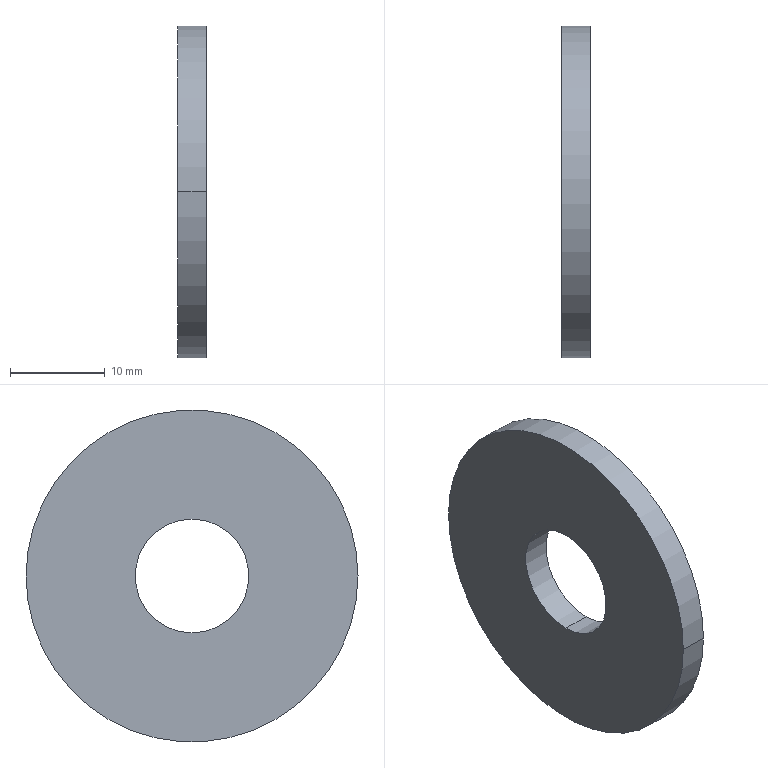Part | STEP file | [02]-15 | 1 solid | 6 faces | box 3 x 35 x 35 mm | volume 2547 mm3 | cylinder 4 | plane 2 | commonest cylinder face diameters 12 x2 35 x2
STEP:
#1=CARTESIAN_POINT('',(0.,0.,0.));
#2=DIRECTION('',(0.,0.,1.));
#3=DIRECTION('',(1.,0.,0.));
#4=AXIS2_PLACEMENT_3D('',#1,#2,#3);
#5=CARTESIAN_POINT('',(0.,0.,-6.));
#6=VERTEX_POINT('',#5);
#7=CARTESIAN_POINT('',(3.,0.,-6.));
#8=VERTEX_POINT('',#7);
#9=CARTESIAN_POINT('',(0.,0.,-6.));
#10=DIRECTION('',(1.,0.,0.));
#11=VECTOR('',#10,1.);
#12=LINE('',#9,#11);
#13=CARTESIAN_POINT('',(0.,0.,0.));
#14=DIRECTION('',(1.,0.,0.));
#15=DIRECTION('',(0.,0.,-1.));
#16=AXIS2_PLACEMENT_3D('',#13,#14,#15);
#17=CYLINDRICAL_SURFACE('',#16,6.);
#18=CARTESIAN_POINT('',(6.283,0.));
#19=DIRECTION('',(0.,1.));
#20=VECTOR('',#19,1.);
#21=LINE('',#18,#20);
#22=(GEOMETRIC_REPRESENTATION_CONTEXT(2)PARAMETRIC_REPRESENTATION_CONTEXT()REPRESENTATION_CONTEXT('',''));
#23=DEFINITIONAL_REPRESENTATION('',(#21),#22);
#24=PCURVE('',#17,#23);
#25=CARTESIAN_POINT('',(0.,0.,0.));
#26=DIRECTION('',(1.,0.,0.));
#27=DIRECTION('',(0.,0.,-1.));
#28=AXIS2_PLACEMENT_3D('',#25,#26,#27);
#29=CYLINDRICAL_SURFACE('',#28,6.);
#30=CARTESIAN_POINT('',(0.,0.));
#31=DIRECTION('',(0.,1.));
#32=VECTOR('',#31,1.);
#33=LINE('',#30,#32);
#34=(GEOMETRIC_REPRESENTATION_CONTEXT(2)PARAMETRIC_REPRESENTATION_CONTEXT()REPRESENTATION_CONTEXT('',''));
#35=DEFINITIONAL_REPRESENTATION('',(#33),#34);
#36=PCURVE('',#29,#35);
#37=SURFACE_CURVE('',#12,(#24,#36),.PCURVE_S1.);
#38=EDGE_CURVE('',#6,#8,#37,.T.);
#39=ORIENTED_EDGE('',*,*,#38,.T.);
#40=CARTESIAN_POINT('',(3.,0.,6.));
#41=VERTEX_POINT('',#40);
#42=CARTESIAN_POINT('',(3.,0.,0.));
#43=DIRECTION('',(-1.,0.,0.));
#44=DIRECTION('',(0.,0.,1.));
#45=AXIS2_PLACEMENT_3D('',#42,#43,#44);
#46=CIRCLE('',#45,6.);
#47=CARTESIAN_POINT('',(9.425,3.));
#48=DIRECTION('',(-1.,0.));
#49=VECTOR('',#48,1.);
#50=LINE('',#47,#49);
#51=(GEOMETRIC_REPRESENTATION_CONTEXT(2)PARAMETRIC_REPRESENTATION_CONTEXT()REPRESENTATION_CONTEXT('',''));
#52=DEFINITIONAL_REPRESENTATION('',(#50),#51);
#53=PCURVE('',#17,#52);
#54=CARTESIAN_POINT('',(3.,0.,0.));
#55=DIRECTION('',(1.,0.,0.));
#56=DIRECTION('',(0.,1.,0.));
#57=AXIS2_PLACEMENT_3D('',#54,#55,#56);
#58=PLANE('',#57);
#59=CARTESIAN_POINT('',(0.,6.));
#60=CARTESIAN_POINT('',(10.392,6.));
#61=CARTESIAN_POINT('',(5.196,-3.));
#62=CARTESIAN_POINT('',(0.,-12.));
#63=CARTESIAN_POINT('',(-5.196,-3.));
#64=CARTESIAN_POINT('',(-10.392,6.));
#65=CARTESIAN_POINT('',(0.,6.));
#66=(BOUNDED_CURVE()B_SPLINE_CURVE(2,(#59,#60,#61,#62,#63,#64,#65),.UNSPECIFIED.,.T.,.F.)B_SPLINE_CURVE_WITH_KNOTS((1,2,2,2,2,1),(-2.094,0.,2.094,4.189,6.283,8.378),.UNSPECIFIED.)CURVE()GEOMETRIC_REPRESENTATION_ITEM()RATIONAL_B_SPLINE_CURVE((1.,0.5,1.,0.5,1.,0.5,1.))REPRESENTATION_ITEM(''));
#67=(GEOMETRIC_REPRESENTATION_CONTEXT(2)PARAMETRIC_REPRESENTATION_CONTEXT()REPRESENTATION_CONTEXT('',''));
#68=DEFINITIONAL_REPRESENTATION('',(#66),#67);
#69=PCURVE('',#58,#68);
#70=SURFACE_CURVE('',#46,(#53,#69),.PCURVE_S1.);
#71=EDGE_CURVE('',#8,#41,#70,.T.);
#72=ORIENTED_EDGE('',*,*,#71,.T.);
#73=CARTESIAN_POINT('',(0.,0.,6.));
#74=VERTEX_POINT('',#73);
#75=CARTESIAN_POINT('',(0.,0.,6.));
#76=DIRECTION('',(1.,0.,0.));
#77=VECTOR('',#76,1.);
#78=LINE('',#75,#77);
#79=CARTESIAN_POINT('',(3.142,0.));
#80=DIRECTION('',(0.,1.));
#81=VECTOR('',#80,1.);
#82=LINE('',#79,#81);
#83=(GEOMETRIC_REPRESENTATION_CONTEXT(2)PARAMETRIC_REPRESENTATION_CONTEXT()REPRESENTATION_CONTEXT('',''));
#84=DEFINITIONAL_REPRESENTATION('',(#82),#83);
#85=PCURVE('',#17,#84);
#86=CARTESIAN_POINT('',(3.142,0.));
#87=DIRECTION('',(0.,1.));
#88=VECTOR('',#87,1.);
#89=LINE('',#86,#88);
#90=(GEOMETRIC_REPRESENTATION_CONTEXT(2)PARAMETRIC_REPRESENTATION_CONTEXT()REPRESENTATION_CONTEXT('',''));
#91=DEFINITIONAL_REPRESENTATION('',(#89),#90);
#92=PCURVE('',#29,#91);
#93=SURFACE_CURVE('',#78,(#85,#92),.PCURVE_S1.);
#94=EDGE_CURVE('',#74,#41,#93,.T.);
#95=ORIENTED_EDGE('',*,*,#94,.F.);
#96=CARTESIAN_POINT('',(0.,0.,0.));
#97=DIRECTION('',(1.,0.,0.));
#98=DIRECTION('',(0.,0.,-1.));
#99=AXIS2_PLACEMENT_3D('',#96,#97,#98);
#100=CIRCLE('',#99,6.);
#101=CARTESIAN_POINT('',(0.,0.));
#102=DIRECTION('',(1.,0.));
#103=VECTOR('',#102,1.);
#104=LINE('',#101,#103);
#105=(GEOMETRIC_REPRESENTATION_CONTEXT(2)PARAMETRIC_REPRESENTATION_CONTEXT()REPRESENTATION_CONTEXT('',''));
#106=DEFINITIONAL_REPRESENTATION('',(#104),#105);
#107=PCURVE('',#17,#106);
#108=CARTESIAN_POINT('',(0.,0.,0.));
#109=DIRECTION('',(-1.,0.,0.));
#110=DIRECTION('',(0.,-1.,0.));
#111=AXIS2_PLACEMENT_3D('',#108,#109,#110);
#112=PLANE('',#111);
#113=CARTESIAN_POINT('',(0.,-6.));
#114=CARTESIAN_POINT('',(-10.392,-6.));
#115=CARTESIAN_POINT('',(-5.196,3.));
#116=CARTESIAN_POINT('',(0.,12.));
#117=CARTESIAN_POINT('',(5.196,3.));
#118=CARTESIAN_POINT('',(10.392,-6.));
#119=CARTESIAN_POINT('',(0.,-6.));
#120=(BOUNDED_CURVE()B_SPLINE_CURVE(2,(#113,#114,#115,#116,#117,#118,#119),.UNSPECIFIED.,.T.,.F.)B_SPLINE_CURVE_WITH_KNOTS((1,2,2,2,2,1),(-2.094,0.,2.094,4.189,6.283,8.378),.UNSPECIFIED.)CURVE()GEOMETRIC_REPRESENTATION_ITEM()RATIONAL_B_SPLINE_CURVE((1.,0.5,1.,0.5,1.,0.5,1.))REPRESENTATION_ITEM(''));
#121=(GEOMETRIC_REPRESENTATION_CONTEXT(2)PARAMETRIC_REPRESENTATION_CONTEXT()REPRESENTATION_CONTEXT('',''));
#122=DEFINITIONAL_REPRESENTATION('',(#120),#121);
#123=PCURVE('',#112,#122);
#124=SURFACE_CURVE('',#100,(#107,#123),.PCURVE_S1.);
#125=EDGE_CURVE('',#74,#6,#124,.T.);
#126=ORIENTED_EDGE('',*,*,#125,.T.);
#127=EDGE_LOOP('',(#39,#72,#95,#126));
#128=FACE_BOUND('',#127,.F.);
#129=ADVANCED_FACE('',(#128),#17,.F.);
#130=CARTESIAN_POINT('',(0.,17.5,0.));
#131=VERTEX_POINT('',#130);
#132=CARTESIAN_POINT('',(0.,-17.5,0.));
#133=VERTEX_POINT('',#132);
#134=CARTESIAN_POINT('',(0.,0.,0.));
#135=DIRECTION('',(1.,0.,0.));
#136=DIRECTION('',(0.,1.,0.));
#137=AXIS2_PLACEMENT_3D('',#134,#135,#136);
#138=CIRCLE('',#137,17.5);
#139=CARTESIAN_POINT('',(0.,0.,0.));
#140=DIRECTION('',(1.,0.,0.));
#141=DIRECTION('',(0.,1.,0.));
#142=AXIS2_PLACEMENT_3D('',#139,#140,#141);
#143=CYLINDRICAL_SURFACE('',#142,17.5);
#144=CARTESIAN_POINT('',(0.,0.));
#145=DIRECTION('',(1.,0.));
#146=VECTOR('',#145,1.);
#147=LINE('',#144,#146);
#148=(GEOMETRIC_REPRESENTATION_CONTEXT(2)PARAMETRIC_REPRESENTATION_CONTEXT()REPRESENTATION_CONTEXT('',''));
#149=DEFINITIONAL_REPRESENTATION('',(#147),#148);
#150=PCURVE('',#143,#149);
#151=CARTESIAN_POINT('',(-17.5,0.));
#152=CARTESIAN_POINT('',(-17.5,30.311));
#153=CARTESIAN_POINT('',(8.75,15.155));
#154=CARTESIAN_POINT('',(35.,0.));
#155=CARTESIAN_POINT('',(8.75,-15.155));
#156=CARTESIAN_POINT('',(-17.5,-30.311));
#157=CARTESIAN_POINT('',(-17.5,0.));
#158=(BOUNDED_CURVE()B_SPLINE_CURVE(2,(#151,#152,#153,#154,#155,#156,#157),.UNSPECIFIED.,.T.,.F.)B_SPLINE_CURVE_WITH_KNOTS((1,2,2,2,2,1),(-2.094,0.,2.094,4.189,6.283,8.378),.UNSPECIFIED.)CURVE()GEOMETRIC_REPRESENTATION_ITEM()RATIONAL_B_SPLINE_CURVE((1.,0.5,1.,0.5,1.,0.5,1.))REPRESENTATION_ITEM(''));
#159=(GEOMETRIC_REPRESENTATION_CONTEXT(2)PARAMETRIC_REPRESENTATION_CONTEXT()REPRESENTATION_CONTEXT('',''));
#160=DEFINITIONAL_REPRESENTATION('',(#158),#159);
#161=PCURVE('',#112,#160);
#162=SURFACE_CURVE('',#138,(#150,#161),.PCURVE_S1.);
#163=EDGE_CURVE('',#131,#133,#162,.T.);
#164=ORIENTED_EDGE('',*,*,#163,.T.);
#165=CARTESIAN_POINT('',(3.,-17.5,0.));
#166=VERTEX_POINT('',#165);
#167=CARTESIAN_POINT('',(0.,-17.5,0.));
#168=DIRECTION('',(1.,0.,0.));
#169=VECTOR('',#168,1.);
#170=LINE('',#167,#169);
#171=CARTESIAN_POINT('',(3.142,0.));
#172=DIRECTION('',(0.,1.));
#173=VECTOR('',#172,1.);
#174=LINE('',#171,#173);
#175=(GEOMETRIC_REPRESENTATION_CONTEXT(2)PARAMETRIC_REPRESENTATION_CONTEXT()REPRESENTATION_CONTEXT('',''));
#176=DEFINITIONAL_REPRESENTATION('',(#174),#175);
#177=PCURVE('',#143,#176);
#178=CARTESIAN_POINT('',(0.,0.,0.));
#179=DIRECTION('',(1.,0.,0.));
#180=DIRECTION('',(0.,1.,0.));
#181=AXIS2_PLACEMENT_3D('',#178,#179,#180);
#182=CYLINDRICAL_SURFACE('',#181,17.5);
#183=CARTESIAN_POINT('',(3.142,0.));
#184=DIRECTION('',(0.,1.));
#185=VECTOR('',#184,1.);
#186=LINE('',#183,#185);
#187=(GEOMETRIC_REPRESENTATION_CONTEXT(2)PARAMETRIC_REPRESENTATION_CONTEXT()REPRESENTATION_CONTEXT('',''));
#188=DEFINITIONAL_REPRESENTATION('',(#186),#187);
#189=PCURVE('',#182,#188);
#190=SURFACE_CURVE('',#170,(#177,#189),.PCURVE_S1.);
#191=EDGE_CURVE('',#133,#166,#190,.T.);
#192=ORIENTED_EDGE('',*,*,#191,.T.);
#193=CARTESIAN_POINT('',(3.,17.5,0.));
#194=VERTEX_POINT('',#193);
#195=CARTESIAN_POINT('',(3.,0.,0.));
#196=DIRECTION('',(-1.,0.,0.));
#197=DIRECTION('',(0.,-1.,0.));
#198=AXIS2_PLACEMENT_3D('',#195,#196,#197);
#199=CIRCLE('',#198,17.5);
#200=CARTESIAN_POINT('',(3.142,3.));
#201=DIRECTION('',(-1.,0.));
#202=VECTOR('',#201,1.);
#203=LINE('',#200,#202);
#204=(GEOMETRIC_REPRESENTATION_CONTEXT(2)PARAMETRIC_REPRESENTATION_CONTEXT()REPRESENTATION_CONTEXT('',''));
#205=DEFINITIONAL_REPRESENTATION('',(#203),#204);
#206=PCURVE('',#143,#205);
#207=CARTESIAN_POINT('',(-17.5,0.));
#208=CARTESIAN_POINT('',(-17.5,30.311));
#209=CARTESIAN_POINT('',(8.75,15.155));
#210=CARTESIAN_POINT('',(35.,0.));
#211=CARTESIAN_POINT('',(8.75,-15.155));
#212=CARTESIAN_POINT('',(-17.5,-30.311));
#213=CARTESIAN_POINT('',(-17.5,0.));
#214=(BOUNDED_CURVE()B_SPLINE_CURVE(2,(#207,#208,#209,#210,#211,#212,#213),.UNSPECIFIED.,.T.,.F.)B_SPLINE_CURVE_WITH_KNOTS((1,2,2,2,2,1),(-2.094,0.,2.094,4.189,6.283,8.378),.UNSPECIFIED.)CURVE()GEOMETRIC_REPRESENTATION_ITEM()RATIONAL_B_SPLINE_CURVE((1.,0.5,1.,0.5,1.,0.5,1.))REPRESENTATION_ITEM(''));
#215=(GEOMETRIC_REPRESENTATION_CONTEXT(2)PARAMETRIC_REPRESENTATION_CONTEXT()REPRESENTATION_CONTEXT('',''));
#216=DEFINITIONAL_REPRESENTATION('',(#214),#215);
#217=PCURVE('',#58,#216);
#218=SURFACE_CURVE('',#199,(#206,#217),.PCURVE_S1.);
#219=EDGE_CURVE('',#166,#194,#218,.T.);
#220=ORIENTED_EDGE('',*,*,#219,.T.);
#221=CARTESIAN_POINT('',(0.,17.5,0.));
#222=DIRECTION('',(1.,0.,0.));
#223=VECTOR('',#222,1.);
#224=LINE('',#221,#223);
#225=CARTESIAN_POINT('',(0.,0.));
#226=DIRECTION('',(0.,1.));
#227=VECTOR('',#226,1.);
#228=LINE('',#225,#227);
#229=(GEOMETRIC_REPRESENTATION_CONTEXT(2)PARAMETRIC_REPRESENTATION_CONTEXT()REPRESENTATION_CONTEXT('',''));
#230=DEFINITIONAL_REPRESENTATION('',(#228),#229);
#231=PCURVE('',#143,#230);
#232=CARTESIAN_POINT('',(6.283,0.));
#233=DIRECTION('',(0.,1.));
#234=VECTOR('',#233,1.);
#235=LINE('',#232,#234);
#236=(GEOMETRIC_REPRESENTATION_CONTEXT(2)PARAMETRIC_REPRESENTATION_CONTEXT()REPRESENTATION_CONTEXT('',''));
#237=DEFINITIONAL_REPRESENTATION('',(#235),#236);
#238=PCURVE('',#182,#237);
#239=SURFACE_CURVE('',#224,(#231,#238),.PCURVE_S1.);
#240=EDGE_CURVE('',#131,#194,#239,.T.);
#241=ORIENTED_EDGE('',*,*,#240,.F.);
#242=EDGE_LOOP('',(#164,#192,#220,#241));
#243=FACE_BOUND('',#242,.T.);
#244=ADVANCED_FACE('',(#243),#143,.T.);
#245=ORIENTED_EDGE('',*,*,#71,.T.);
#246=CARTESIAN_POINT('',(3.,0.,0.));
#247=DIRECTION('',(-1.,0.,0.));
#248=DIRECTION('',(0.,0.,1.));
#249=AXIS2_PLACEMENT_3D('',#246,#247,#248);
#250=CIRCLE('',#249,6.);
#251=CARTESIAN_POINT('',(0.,6.));
#252=CARTESIAN_POINT('',(10.392,6.));
#253=CARTESIAN_POINT('',(5.196,-3.));
#254=CARTESIAN_POINT('',(0.,-12.));
#255=CARTESIAN_POINT('',(-5.196,-3.));
#256=CARTESIAN_POINT('',(-10.392,6.));
#257=CARTESIAN_POINT('',(0.,6.));
#258=(BOUNDED_CURVE()B_SPLINE_CURVE(2,(#251,#252,#253,#254,#255,#256,#257),.UNSPECIFIED.,.T.,.F.)B_SPLINE_CURVE_WITH_KNOTS((1,2,2,2,2,1),(-2.094,0.,2.094,4.189,6.283,8.378),.UNSPECIFIED.)CURVE()GEOMETRIC_REPRESENTATION_ITEM()RATIONAL_B_SPLINE_CURVE((1.,0.5,1.,0.5,1.,0.5,1.))REPRESENTATION_ITEM(''));
#259=(GEOMETRIC_REPRESENTATION_CONTEXT(2)PARAMETRIC_REPRESENTATION_CONTEXT()REPRESENTATION_CONTEXT('',''));
#260=DEFINITIONAL_REPRESENTATION('',(#258),#259);
#261=PCURVE('',#58,#260);
#262=CARTESIAN_POINT('',(3.142,3.));
#263=DIRECTION('',(-1.,0.));
#264=VECTOR('',#263,1.);
#265=LINE('',#262,#264);
#266=(GEOMETRIC_REPRESENTATION_CONTEXT(2)PARAMETRIC_REPRESENTATION_CONTEXT()REPRESENTATION_CONTEXT('',''));
#267=DEFINITIONAL_REPRESENTATION('',(#265),#266);
#268=PCURVE('',#29,#267);
#269=SURFACE_CURVE('',#250,(#261,#268),.PCURVE_S1.);
#270=EDGE_CURVE('',#41,#8,#269,.T.);
#271=ORIENTED_EDGE('',*,*,#270,.T.);
#272=EDGE_LOOP('',(#245,#271));
#273=FACE_BOUND('',#272,.T.);
#274=CARTESIAN_POINT('',(3.,0.,0.));
#275=DIRECTION('',(-1.,0.,0.));
#276=DIRECTION('',(0.,-1.,0.));
#277=AXIS2_PLACEMENT_3D('',#274,#275,#276);
#278=CIRCLE('',#277,17.5);
#279=CARTESIAN_POINT('',(-17.5,0.));
#280=CARTESIAN_POINT('',(-17.5,30.311));
#281=CARTESIAN_POINT('',(8.75,15.155));
#282=CARTESIAN_POINT('',(35.,0.));
#283=CARTESIAN_POINT('',(8.75,-15.155));
#284=CARTESIAN_POINT('',(-17.5,-30.311));
#285=CARTESIAN_POINT('',(-17.5,0.));
#286=(BOUNDED_CURVE()B_SPLINE_CURVE(2,(#279,#280,#281,#282,#283,#284,#285),.UNSPECIFIED.,.T.,.F.)B_SPLINE_CURVE_WITH_KNOTS((1,2,2,2,2,1),(-2.094,0.,2.094,4.189,6.283,8.378),.UNSPECIFIED.)CURVE()GEOMETRIC_REPRESENTATION_ITEM()RATIONAL_B_SPLINE_CURVE((1.,0.5,1.,0.5,1.,0.5,1.))REPRESENTATION_ITEM(''));
#287=(GEOMETRIC_REPRESENTATION_CONTEXT(2)PARAMETRIC_REPRESENTATION_CONTEXT()REPRESENTATION_CONTEXT('',''));
#288=DEFINITIONAL_REPRESENTATION('',(#286),#287);
#289=PCURVE('',#58,#288);
#290=CARTESIAN_POINT('',(9.425,3.));
#291=DIRECTION('',(-1.,0.));
#292=VECTOR('',#291,1.);
#293=LINE('',#290,#292);
#294=(GEOMETRIC_REPRESENTATION_CONTEXT(2)PARAMETRIC_REPRESENTATION_CONTEXT()REPRESENTATION_CONTEXT('',''));
#295=DEFINITIONAL_REPRESENTATION('',(#293),#294);
#296=PCURVE('',#182,#295);
#297=SURFACE_CURVE('',#278,(#289,#296),.PCURVE_S1.);
#298=EDGE_CURVE('',#194,#166,#297,.T.);
#299=ORIENTED_EDGE('',*,*,#298,.F.);
#300=ORIENTED_EDGE('',*,*,#219,.F.);
#301=EDGE_LOOP('',(#299,#300));
#302=FACE_BOUND('',#301,.T.);
#303=ADVANCED_FACE('',(#273,#302),#58,.T.);
#304=CARTESIAN_POINT('',(0.,0.,0.));
#305=DIRECTION('',(1.,0.,0.));
#306=DIRECTION('',(0.,0.,-1.));
#307=AXIS2_PLACEMENT_3D('',#304,#305,#306);
#308=CIRCLE('',#307,6.);
#309=CARTESIAN_POINT('',(0.,-6.));
#310=CARTESIAN_POINT('',(-10.392,-6.));
#311=CARTESIAN_POINT('',(-5.196,3.));
#312=CARTESIAN_POINT('',(0.,12.));
#313=CARTESIAN_POINT('',(5.196,3.));
#314=CARTESIAN_POINT('',(10.392,-6.));
#315=CARTESIAN_POINT('',(0.,-6.));
#316=(BOUNDED_CURVE()B_SPLINE_CURVE(2,(#309,#310,#311,#312,#313,#314,#315),.UNSPECIFIED.,.T.,.F.)B_SPLINE_CURVE_WITH_KNOTS((1,2,2,2,2,1),(-2.094,0.,2.094,4.189,6.283,8.378),.UNSPECIFIED.)CURVE()GEOMETRIC_REPRESENTATION_ITEM()RATIONAL_B_SPLINE_CURVE((1.,0.5,1.,0.5,1.,0.5,1.))REPRESENTATION_ITEM(''));
#317=(GEOMETRIC_REPRESENTATION_CONTEXT(2)PARAMETRIC_REPRESENTATION_CONTEXT()REPRESENTATION_CONTEXT('',''));
#318=DEFINITIONAL_REPRESENTATION('',(#316),#317);
#319=PCURVE('',#112,#318);
#320=CARTESIAN_POINT('',(0.,0.));
#321=DIRECTION('',(1.,0.));
#322=VECTOR('',#321,1.);
#323=LINE('',#320,#322);
#324=(GEOMETRIC_REPRESENTATION_CONTEXT(2)PARAMETRIC_REPRESENTATION_CONTEXT()REPRESENTATION_CONTEXT('',''));
#325=DEFINITIONAL_REPRESENTATION('',(#323),#324);
#326=PCURVE('',#29,#325);
#327=SURFACE_CURVE('',#308,(#319,#326),.PCURVE_S1.);
#328=EDGE_CURVE('',#6,#74,#327,.T.);
#329=ORIENTED_EDGE('',*,*,#328,.T.);
#330=ORIENTED_EDGE('',*,*,#125,.T.);
#331=EDGE_LOOP('',(#329,#330));
#332=FACE_BOUND('',#331,.T.);
#333=ORIENTED_EDGE('',*,*,#163,.F.);
#334=CARTESIAN_POINT('',(0.,0.,0.));
#335=DIRECTION('',(1.,0.,0.));
#336=DIRECTION('',(0.,1.,0.));
#337=AXIS2_PLACEMENT_3D('',#334,#335,#336);
#338=CIRCLE('',#337,17.5);
#339=CARTESIAN_POINT('',(-17.5,0.));
#340=CARTESIAN_POINT('',(-17.5,30.311));
#341=CARTESIAN_POINT('',(8.75,15.155));
#342=CARTESIAN_POINT('',(35.,0.));
#343=CARTESIAN_POINT('',(8.75,-15.155));
#344=CARTESIAN_POINT('',(-17.5,-30.311));
#345=CARTESIAN_POINT('',(-17.5,0.));
#346=(BOUNDED_CURVE()B_SPLINE_CURVE(2,(#339,#340,#341,#342,#343,#344,#345),.UNSPECIFIED.,.T.,.F.)B_SPLINE_CURVE_WITH_KNOTS((1,2,2,2,2,1),(-2.094,0.,2.094,4.189,6.283,8.378),.UNSPECIFIED.)CURVE()GEOMETRIC_REPRESENTATION_ITEM()RATIONAL_B_SPLINE_CURVE((1.,0.5,1.,0.5,1.,0.5,1.))REPRESENTATION_ITEM(''));
#347=(GEOMETRIC_REPRESENTATION_CONTEXT(2)PARAMETRIC_REPRESENTATION_CONTEXT()REPRESENTATION_CONTEXT('',''));
#348=DEFINITIONAL_REPRESENTATION('',(#346),#347);
#349=PCURVE('',#112,#348);
#350=CARTESIAN_POINT('',(0.,0.));
#351=DIRECTION('',(1.,0.));
#352=VECTOR('',#351,1.);
#353=LINE('',#350,#352);
#354=(GEOMETRIC_REPRESENTATION_CONTEXT(2)PARAMETRIC_REPRESENTATION_CONTEXT()REPRESENTATION_CONTEXT('',''));
#355=DEFINITIONAL_REPRESENTATION('',(#353),#354);
#356=PCURVE('',#182,#355);
#357=SURFACE_CURVE('',#338,(#349,#356),.PCURVE_S1.);
#358=EDGE_CURVE('',#133,#131,#357,.T.);
#359=ORIENTED_EDGE('',*,*,#358,.F.);
#360=EDGE_LOOP('',(#333,#359));
#361=FACE_BOUND('',#360,.T.);
#362=ADVANCED_FACE('',(#332,#361),#112,.T.);
#363=ORIENTED_EDGE('',*,*,#191,.F.);
#364=ORIENTED_EDGE('',*,*,#358,.T.);
#365=ORIENTED_EDGE('',*,*,#240,.T.);
#366=ORIENTED_EDGE('',*,*,#298,.T.);
#367=EDGE_LOOP('',(#363,#364,#365,#366));
#368=FACE_BOUND('',#367,.T.);
#369=ADVANCED_FACE('',(#368),#182,.T.);
#370=ORIENTED_EDGE('',*,*,#270,.T.);
#371=ORIENTED_EDGE('',*,*,#38,.F.);
#372=ORIENTED_EDGE('',*,*,#328,.T.);
#373=ORIENTED_EDGE('',*,*,#94,.T.);
#374=EDGE_LOOP('',(#370,#371,#372,#373));
#375=FACE_BOUND('',#374,.F.);
#376=ADVANCED_FACE('',(#375),#29,.F.);
#377=CLOSED_SHELL('',(#129,#244,#303,#362,#369,#376));
#378=MANIFOLD_SOLID_BREP('',#377);
#379=(LENGTH_UNIT()NAMED_UNIT(*)SI_UNIT(.MILLI.,.METRE.));
#380=UNCERTAINTY_MEASURE_WITH_UNIT(LENGTH_MEASURE(0.0000001),#379,'','');
#381=(NAMED_UNIT(*)PLANE_ANGLE_UNIT()SI_UNIT($,.RADIAN.));
#382=(NAMED_UNIT(*)SI_UNIT($,.STERADIAN.)SOLID_ANGLE_UNIT());
#383=(GEOMETRIC_REPRESENTATION_CONTEXT(3)GLOBAL_UNCERTAINTY_ASSIGNED_CONTEXT((#380))GLOBAL_UNIT_ASSIGNED_CONTEXT((#379,#381,#382))REPRESENTATION_CONTEXT('',''));
#384=ADVANCED_BREP_SHAPE_REPRESENTATION('',(#4,#378),#383);